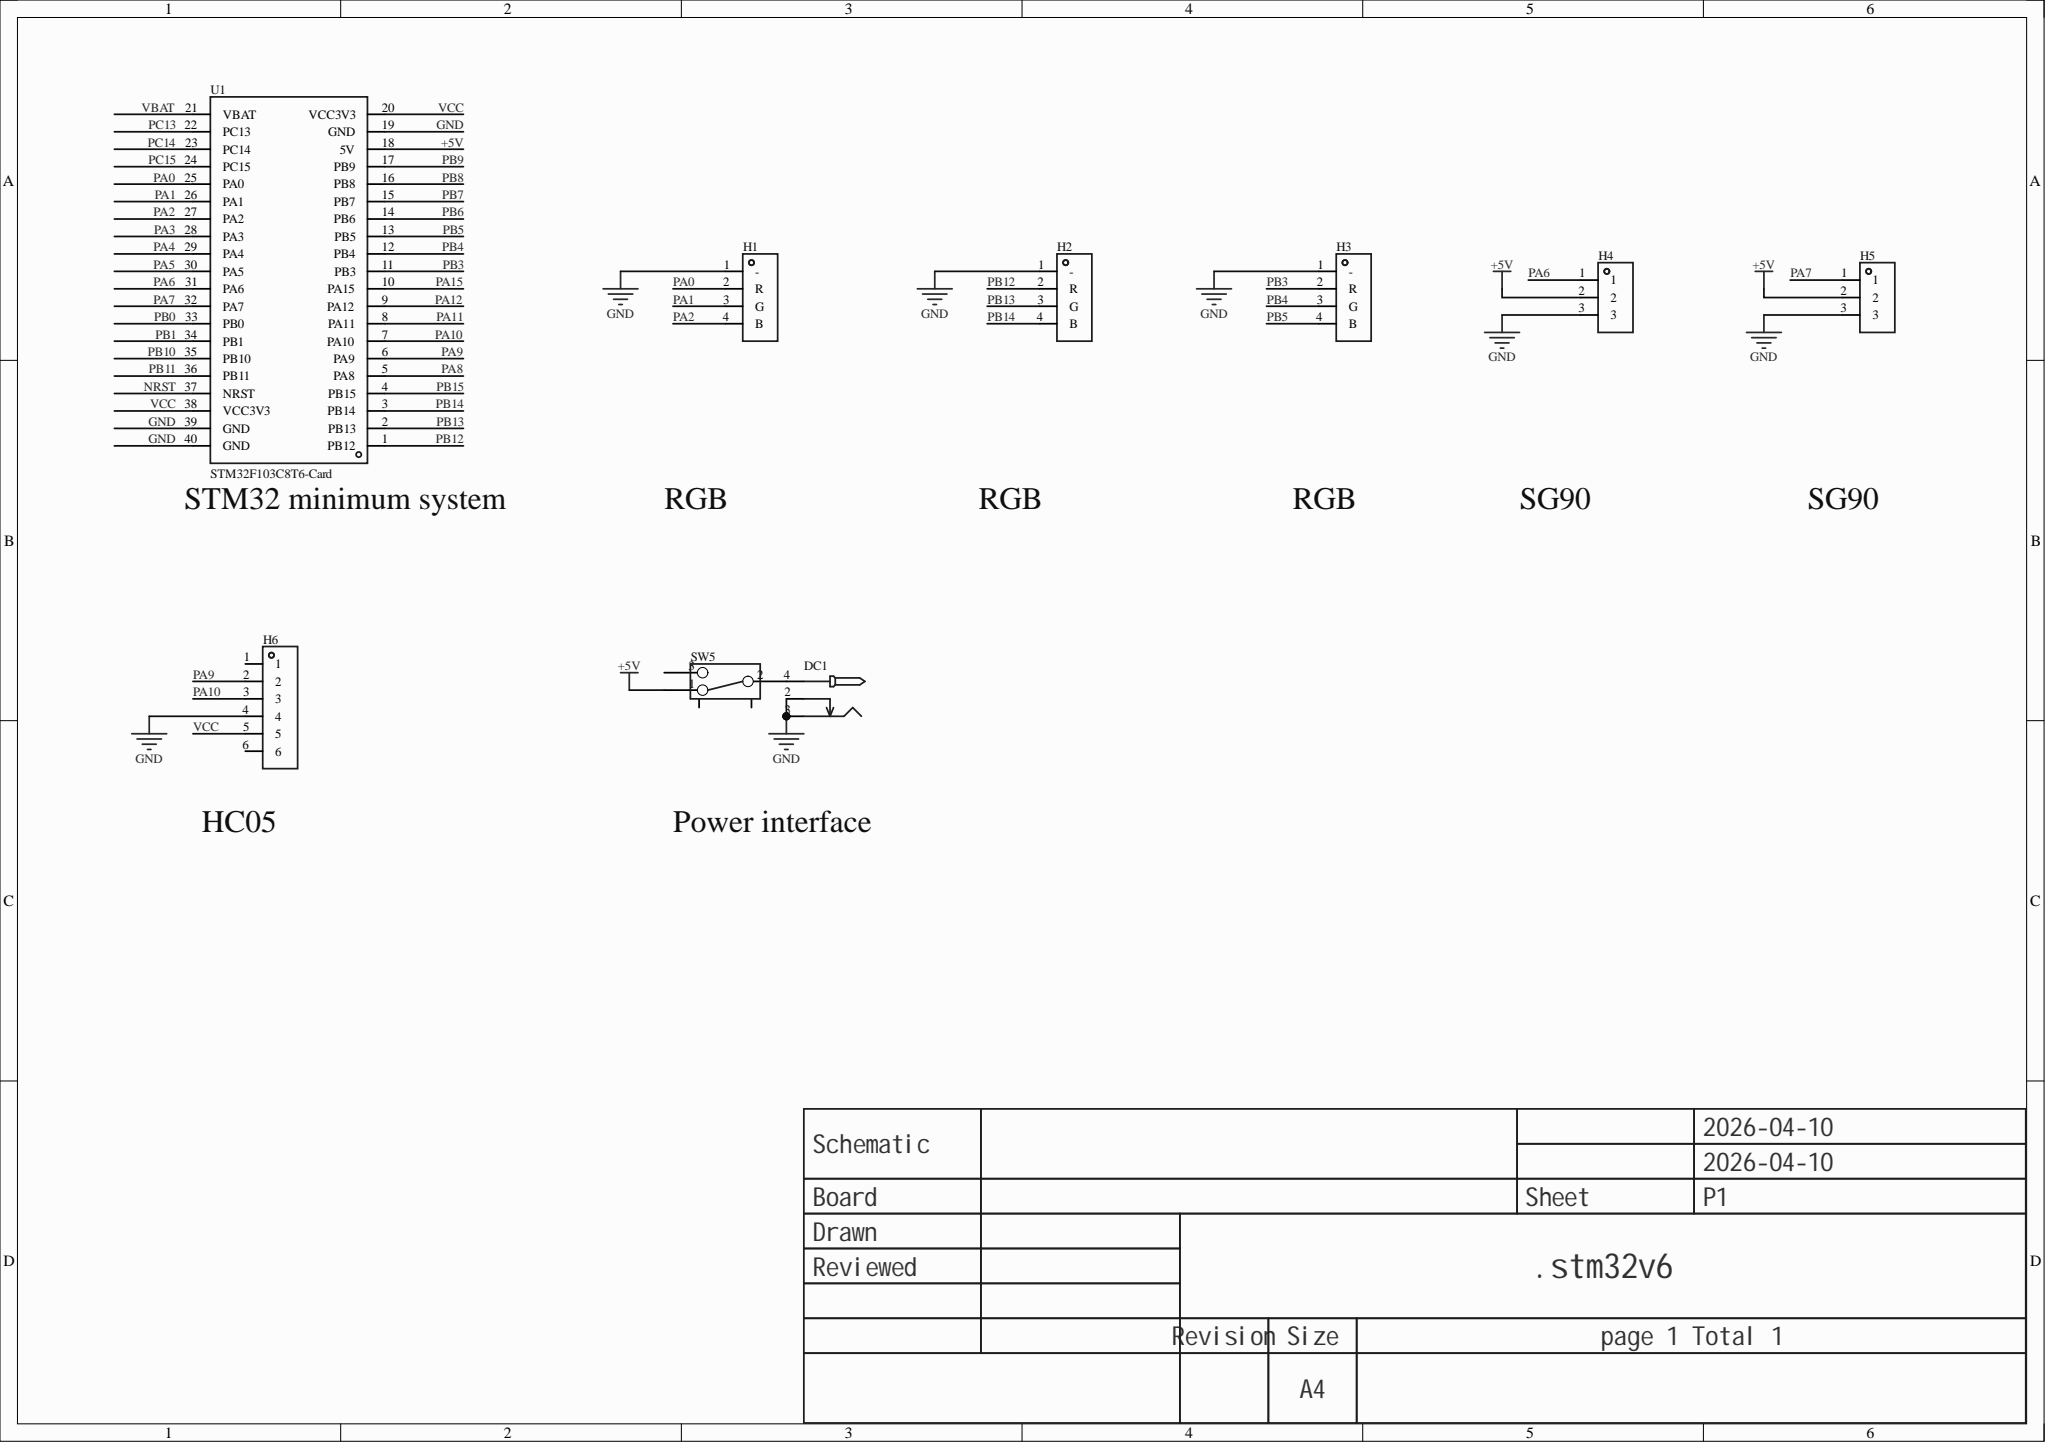Circuit board | Altium Designer | 9 parts | 17 nets
Bill of materials:
Comment,Description,Designator,Footprint,LibRef,Quantity
"","","DC1","DC-2.0","DC-005_2.0","1"
"","","H1, H2, H3","HDR-TH_4P-P2.54-V-F","HDR-F_2.54_1x4P","3"
"","","H4, H5","HDR-TH_3P-P2.54-V-M","HDR-M_2.54_1x3P","2"
"","","H6","HDR-TH_6P-P2.54-V-F","HDR-F_2.54_1x6P","1"
"","","SW5","拨动开关","拨动开关_正","1"
"STM32F103C8T6-Card","","U1","CONN-TH_L53.3-W22.9_STM32F103C8T6-CARD","STM32F103C8T6-Card","1"
Netlist (Protel format):
[
DC1
DC-2.0




]
[
H1
HDR-TH_4P-P2.54-V-F




]
[
H2
HDR-TH_4P-P2.54-V-F




]
[
H3
HDR-TH_4P-P2.54-V-F




]
[
H4
HDR-TH_3P-P2.54-V-M




]
[
H5
HDR-TH_3P-P2.54-V-M




]
[
H6
HDR-TH_6P-P2.54-V-F




]
[
SW5
拨动开关




]
[
U1
CONN-TH_L53.3-W22.9_STM32F103C8T6-CARD
STM32F103C8T6-Card



]
(
VCC
H6-5
U1-20
U1-38
)
(
PB14
H2-4
U1-3
)
(
PB13
H2-3
U1-2
)
(
PB12
H2-2
U1-1
)
(
PB5
H3-4
U1-13
)
(
PB4
H3-3
U1-12
)
(
PB3
H3-2
U1-11
)
(
PA10
H6-3
U1-7
)
(
PA9
H6-2
U1-6
)
(
PA7
H5-1
U1-32
)
(
PA6
H4-1
U1-31
)
(
PA2
H1-4
U1-27
)
(
PA1
H1-3
U1-26
)
(
PA0
H1-2
U1-25
)
(
NetDC1_4
DC1-4
SW5-2
)
(
GND
DC1-2
DC1-3
H1-1
H2-1
H3-1
H4-3
H5-3
H6-4
U1-19
U1-39
U1-40
)
(
+5V
H4-2
H5-2
SW5-1
U1-18
)